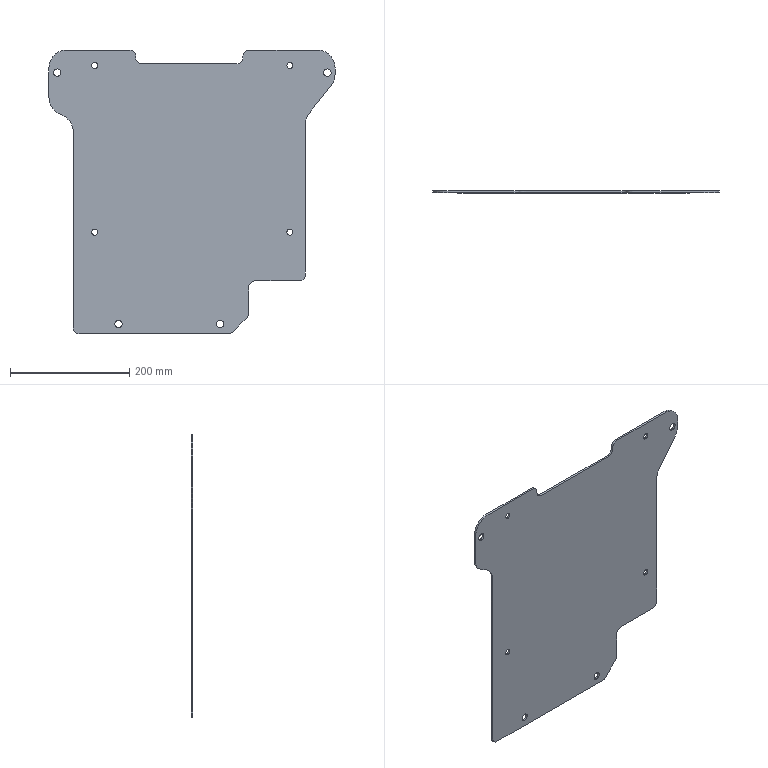Part | SolidWorks | features FlatPattern 1, SMBaseFlange 1, SheetMetal 1 | 1 solid | 48 faces | box 481 x 3.2 x 477 mm | volume 577173 mm3 | cylinder 31 | plane 17 | commonest cylinder face diameters 20 x9 10 x8 12.5 x8 60 x6